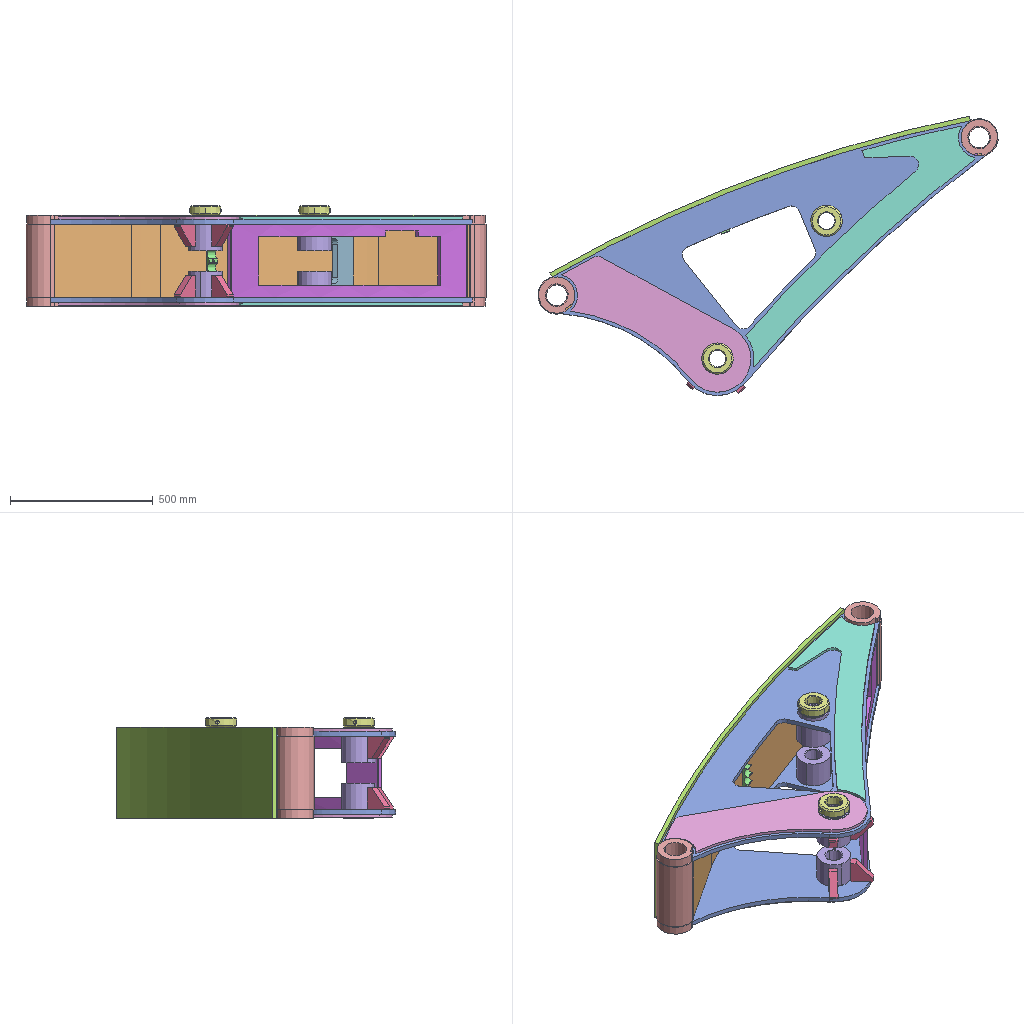Assembly | SolidWorks | 12 different items | 23 placed | box 1613 x 980 x 354 mm
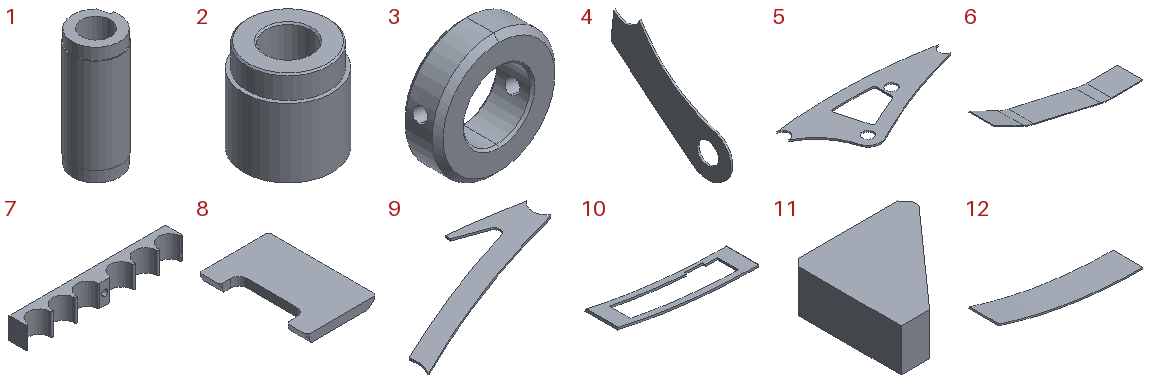Parts list (item | quantity | size | volume | features):
1 | x2 | 133 x 133 x 320 mm | 2826163 mm3 | features ICE 3, Extrusion 1, MirrorPattern 1
2 | x4 | 120 x 120 x 124 mm | 994353 mm3 | features Chamfer 1, Extrusion 1, ICE 1
3 | x2 | 110 x 34 x 110 mm | 211578 mm3 | features Chamfer 2, 3DProfileFeature 1, Extrusion 1, HoleWzd 1
4 | x2 | 10 x 612.332 x 532.004 mm | 1222648 mm3 | features Extrusion 1
5 | x2 | 1582 x 654.084 x 16 mm | 7594326 mm3 | features Extrusion 1
6 | x1 | 1515 x 258 x 356.966 mm | 3243782 mm3 | features SM3dBend 2, FlatPattern 1, SMBaseFlange 1, SheetMetal 1
7 | x1 | 214 x 25 x 30 mm | 86293 mm3 | features Extrusion 1, HoleWzd 1
8 | x1 | 166 x 258 x 20 mm | 651811 mm3 | features Extrusion 1, ICE 1
9 | x2 | 997.777 x 556.587 x 10 mm | 1190658 mm3 | features Extrusion 1
10 | x1 | 1142 x 258 x 145.694 mm | 2305600 mm3 | features FlatPattern 1, SM3dBend 1, SMBaseFlange 1, SheetMetal 1
11 | x4 | 80 x 77.5 x 30 mm | 124500 mm3 | features Extrusion 1
12 | x1 | 1551 x 320 x 260.824 mm | 8058880 mm3 | features FlatPattern 1, SM3dBend 1, SMBaseFlange 1, SheetMetal 1
Mates (type | each side: item.copy, entity, surface, feature):
Concentric | 1.1 face cylinder Mirror1 | 5.1 face cylinder Boss-Extrude1
Coincident | 1.1 face plane Mirror1 | 5.1 face plane Boss-Extrude1
Concentric | 5.1 face cylinder Boss-Extrude1 | 12.1 face cylinder Sketch Bend1
Coincident | 1.1 face cylinder Boss-Extrude1 | 12.1 edge
Concentric | 5.2 face cylinder Boss-Extrude1 | 4.1 face cylinder Boss-Extrude1
Concentric | 1.1 face cylinder Cut-Extrude2 | 4.1 face cylinder Boss-Extrude1
Coincident | 5.2 face plane Boss-Extrude1 | 4.1 face plane Boss-Extrude1
Concentric | 5.2 face cylinder Boss-Extrude1 | 9.1 face cylinder Boss-Extrude1
Concentric | 4.1 face cylinder Boss-Extrude1 | 9.1 face cylinder Boss-Extrude1
Coincident | 5.2 face plane Boss-Extrude1 | 9.1 face plane Boss-Extrude1
Concentric | 5.2 face cylinder Boss-Extrude1 | 1.2 face cylinder Cut-Extrude1
Coincident | 5.2 face plane Boss-Extrude1 | 1.2 face plane Mirror1
Coincident | 5.2 face plane Boss-Extrude1 | 6.1 face plane Base-Flange1
Coincident | 1.2 face plane Cut-Extrude3 | 6.1 face plane Base-Flange1
Coincident | 1.1 face plane Cut-Extrude3 | 6.1 face plane Sketched Bend3
Coincident | 1.1 face plane Cut-Extrude3 | 6.1 edge
Concentric | 5.2 face cylinder Boss-Extrude1 | 2.1 face cylinder Cut-Extrude1
Coincident | 5.2 face plane Boss-Extrude1 | 2.1 face plane Cut-Extrude1
Concentric | 5.1 face cylinder Boss-Extrude1 | 2.2 face cylinder Boss-Extrude1
Coincident | 5.1 face plane Boss-Extrude1 | 2.2 face plane Cut-Extrude1
Concentric | 5.2 face cylinder Boss-Extrude1 | 2.3 face cylinder Boss-Extrude1
Coincident | 5.2 face plane Boss-Extrude1 | 2.3 face plane Cut-Extrude1
Concentric | 5.1 face cylinder Boss-Extrude1 | 2.4 face cylinder Boss-Extrude1
Coincident | 5.1 face plane Boss-Extrude1 | 2.4 face plane Cut-Extrude1
Coincident | 12.1 face plane Sketch Bend1 | 1.2 face plane Boss-Extrude1
DistanceDim | 7.1 face plane Boss-Extrude1 | 1.1 face plane Boss-Extrude1
DistanceDim | 7.1 face plane Boss-Extrude1 | 12.1 vertex
Coincident | 6.1 face plane Sketched Bend4 | 7.1 face plane Boss-Extrude1
Coincident | 5.1 face plane Boss-Extrude1 | 11.1 face plane Boss-Extrude1
Coincident | 5.1 face plane Boss-Extrude1 | 11.2 face plane Boss-Extrude1
Tangent | 2.2 face cylinder Boss-Extrude1 | 11.1 face plane Boss-Extrude1
Coincident | 5.1 vertex | 11.1 edge
Tangent | 2.2 face cylinder Boss-Extrude1 | 11.2 face plane Boss-Extrude1
Lock | 2.2 select_type:0 | 11.1 select_type:0
Lock | 2.2 select_type:0 | 11.2 select_type:0
Coincident | 5.1 face plane Boss-Extrude1 | 8.1 face plane Boss-Extrude1
Coincident | 6.1 face plane Sketched Bend4 | 8.1 face plane Cut-Extrude1
Tangent | 2.4 face cylinder Boss-Extrude1 | 8.1 face plane Cut-Extrude1
Concentric | 2.1 face cylinder Boss-Extrude1 | 3.1 face cylinder Boss-Extrude1
Coincident | 2.1 face plane Boss-Extrude1 | 3.1 face plane Boss-Extrude1
Concentric | 2.3 face cylinder Boss-Extrude1 | 3.2 face cylinder Boss-Extrude1
Coincident | 2.3 face plane Boss-Extrude1 | 3.2 face plane Boss-Extrude1
Concentric | 10.1 face cylinder Sketch Bend1 | 5.2 face cylinder Boss-Extrude1
Coincident | 10.1 face plane Sketch Bend1 | 5.2 face plane Boss-Extrude1
Coincident | 1.2 face cylinder Boss-Extrude1 | 10.1 edge